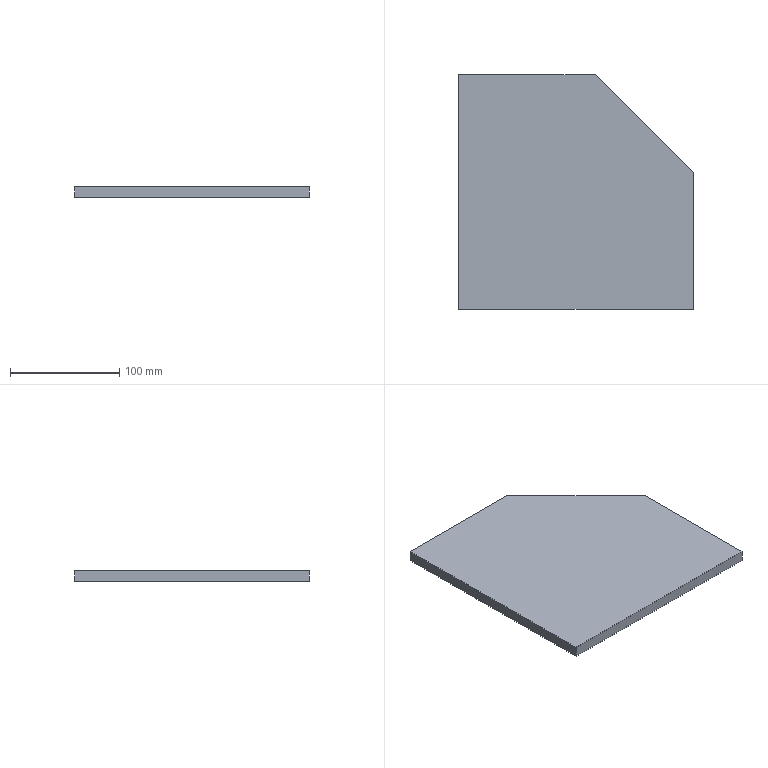Part | STEP file | 03-Reinforcing rib plate | 1 solid | 7 faces | box 215 x 215 x 10 mm | volume 421750 mm3 | plane 7
STEP:
#1=CARTESIAN_POINT('',(0.,0.,0.));
#2=DIRECTION('',(0.,0.,1.));
#3=DIRECTION('',(1.,0.,0.));
#4=AXIS2_PLACEMENT_3D('',#1,#2,#3);
#5=CARTESIAN_POINT('',(0.,0.,0.));
#6=VERTEX_POINT('',#5);
#7=CARTESIAN_POINT('',(0.,-215.,0.));
#8=VERTEX_POINT('',#7);
#9=CARTESIAN_POINT('',(0.,0.,0.));
#10=DIRECTION('',(0.,-1.,0.));
#11=VECTOR('',#10,1.);
#12=LINE('',#9,#11);
#13=CARTESIAN_POINT('',(0.,0.,10.));
#14=DIRECTION('',(1.,0.,0.));
#15=DIRECTION('',(0.,1.,0.));
#16=AXIS2_PLACEMENT_3D('',#13,#14,#15);
#17=PLANE('',#16);
#18=CARTESIAN_POINT('',(0.,-10.));
#19=DIRECTION('',(-1.,0.));
#20=VECTOR('',#19,1.);
#21=LINE('',#18,#20);
#22=(GEOMETRIC_REPRESENTATION_CONTEXT(2)PARAMETRIC_REPRESENTATION_CONTEXT()REPRESENTATION_CONTEXT('',''));
#23=DEFINITIONAL_REPRESENTATION('',(#21),#22);
#24=PCURVE('',#17,#23);
#25=CARTESIAN_POINT('',(0.,0.,0.));
#26=DIRECTION('',(0.,0.,1.));
#27=DIRECTION('',(1.,0.,0.));
#28=AXIS2_PLACEMENT_3D('',#25,#26,#27);
#29=PLANE('',#28);
#30=CARTESIAN_POINT('',(0.,0.));
#31=DIRECTION('',(0.,-1.));
#32=VECTOR('',#31,1.);
#33=LINE('',#30,#32);
#34=(GEOMETRIC_REPRESENTATION_CONTEXT(2)PARAMETRIC_REPRESENTATION_CONTEXT()REPRESENTATION_CONTEXT('',''));
#35=DEFINITIONAL_REPRESENTATION('',(#33),#34);
#36=PCURVE('',#29,#35);
#37=SURFACE_CURVE('',#12,(#24,#36),.PCURVE_S1.);
#38=EDGE_CURVE('',#6,#8,#37,.T.);
#39=ORIENTED_EDGE('',*,*,#38,.T.);
#40=CARTESIAN_POINT('',(0.,-215.,10.));
#41=VERTEX_POINT('',#40);
#42=CARTESIAN_POINT('',(0.,-215.,10.));
#43=DIRECTION('',(0.,0.,-1.));
#44=VECTOR('',#43,1.);
#45=LINE('',#42,#44);
#46=CARTESIAN_POINT('',(-215.,0.));
#47=DIRECTION('',(0.,-1.));
#48=VECTOR('',#47,1.);
#49=LINE('',#46,#48);
#50=(GEOMETRIC_REPRESENTATION_CONTEXT(2)PARAMETRIC_REPRESENTATION_CONTEXT()REPRESENTATION_CONTEXT('',''));
#51=DEFINITIONAL_REPRESENTATION('',(#49),#50);
#52=PCURVE('',#17,#51);
#53=CARTESIAN_POINT('',(0.,-215.,10.));
#54=DIRECTION('',(0.,1.,0.));
#55=DIRECTION('',(0.,0.,1.));
#56=AXIS2_PLACEMENT_3D('',#53,#54,#55);
#57=PLANE('',#56);
#58=CARTESIAN_POINT('',(0.,0.));
#59=DIRECTION('',(-1.,0.));
#60=VECTOR('',#59,1.);
#61=LINE('',#58,#60);
#62=(GEOMETRIC_REPRESENTATION_CONTEXT(2)PARAMETRIC_REPRESENTATION_CONTEXT()REPRESENTATION_CONTEXT('',''));
#63=DEFINITIONAL_REPRESENTATION('',(#61),#62);
#64=PCURVE('',#57,#63);
#65=SURFACE_CURVE('',#45,(#52,#64),.PCURVE_S1.);
#66=EDGE_CURVE('',#41,#8,#65,.T.);
#67=ORIENTED_EDGE('',*,*,#66,.F.);
#68=CARTESIAN_POINT('',(0.,0.,10.));
#69=VERTEX_POINT('',#68);
#70=CARTESIAN_POINT('',(0.,0.,10.));
#71=DIRECTION('',(0.,-1.,0.));
#72=VECTOR('',#71,1.);
#73=LINE('',#70,#72);
#74=CARTESIAN_POINT('',(0.,0.));
#75=DIRECTION('',(-1.,0.));
#76=VECTOR('',#75,1.);
#77=LINE('',#74,#76);
#78=(GEOMETRIC_REPRESENTATION_CONTEXT(2)PARAMETRIC_REPRESENTATION_CONTEXT()REPRESENTATION_CONTEXT('',''));
#79=DEFINITIONAL_REPRESENTATION('',(#77),#78);
#80=PCURVE('',#17,#79);
#81=CARTESIAN_POINT('',(0.,0.,10.));
#82=DIRECTION('',(0.,0.,1.));
#83=DIRECTION('',(1.,0.,0.));
#84=AXIS2_PLACEMENT_3D('',#81,#82,#83);
#85=PLANE('',#84);
#86=CARTESIAN_POINT('',(0.,0.));
#87=DIRECTION('',(0.,-1.));
#88=VECTOR('',#87,1.);
#89=LINE('',#86,#88);
#90=(GEOMETRIC_REPRESENTATION_CONTEXT(2)PARAMETRIC_REPRESENTATION_CONTEXT()REPRESENTATION_CONTEXT('',''));
#91=DEFINITIONAL_REPRESENTATION('',(#89),#90);
#92=PCURVE('',#85,#91);
#93=SURFACE_CURVE('',#73,(#80,#92),.PCURVE_S1.);
#94=EDGE_CURVE('',#69,#41,#93,.T.);
#95=ORIENTED_EDGE('',*,*,#94,.F.);
#96=CARTESIAN_POINT('',(0.,0.,10.));
#97=DIRECTION('',(0.,0.,-1.));
#98=VECTOR('',#97,1.);
#99=LINE('',#96,#98);
#100=CARTESIAN_POINT('',(0.,0.));
#101=DIRECTION('',(0.,-1.));
#102=VECTOR('',#101,1.);
#103=LINE('',#100,#102);
#104=(GEOMETRIC_REPRESENTATION_CONTEXT(2)PARAMETRIC_REPRESENTATION_CONTEXT()REPRESENTATION_CONTEXT('',''));
#105=DEFINITIONAL_REPRESENTATION('',(#103),#104);
#106=PCURVE('',#17,#105);
#107=CARTESIAN_POINT('',(0.,0.,10.));
#108=DIRECTION('',(0.,-1.,0.));
#109=DIRECTION('',(0.,0.,-1.));
#110=AXIS2_PLACEMENT_3D('',#107,#108,#109);
#111=PLANE('',#110);
#112=CARTESIAN_POINT('',(0.,0.));
#113=DIRECTION('',(1.,0.));
#114=VECTOR('',#113,1.);
#115=LINE('',#112,#114);
#116=(GEOMETRIC_REPRESENTATION_CONTEXT(2)PARAMETRIC_REPRESENTATION_CONTEXT()REPRESENTATION_CONTEXT('',''));
#117=DEFINITIONAL_REPRESENTATION('',(#115),#116);
#118=PCURVE('',#111,#117);
#119=SURFACE_CURVE('',#99,(#106,#118),.PCURVE_S1.);
#120=EDGE_CURVE('',#69,#6,#119,.T.);
#121=ORIENTED_EDGE('',*,*,#120,.T.);
#122=EDGE_LOOP('',(#39,#67,#95,#121));
#123=FACE_BOUND('',#122,.T.);
#124=ADVANCED_FACE('',(#123),#17,.F.);
#125=CARTESIAN_POINT('',(215.,-215.,0.));
#126=VERTEX_POINT('',#125);
#127=CARTESIAN_POINT('',(0.,-215.,0.));
#128=DIRECTION('',(1.,0.,0.));
#129=VECTOR('',#128,1.);
#130=LINE('',#127,#129);
#131=CARTESIAN_POINT('',(-10.,0.));
#132=DIRECTION('',(0.,1.));
#133=VECTOR('',#132,1.);
#134=LINE('',#131,#133);
#135=(GEOMETRIC_REPRESENTATION_CONTEXT(2)PARAMETRIC_REPRESENTATION_CONTEXT()REPRESENTATION_CONTEXT('',''));
#136=DEFINITIONAL_REPRESENTATION('',(#134),#135);
#137=PCURVE('',#57,#136);
#138=CARTESIAN_POINT('',(0.,-215.));
#139=DIRECTION('',(1.,0.));
#140=VECTOR('',#139,1.);
#141=LINE('',#138,#140);
#142=(GEOMETRIC_REPRESENTATION_CONTEXT(2)PARAMETRIC_REPRESENTATION_CONTEXT()REPRESENTATION_CONTEXT('',''));
#143=DEFINITIONAL_REPRESENTATION('',(#141),#142);
#144=PCURVE('',#29,#143);
#145=SURFACE_CURVE('',#130,(#137,#144),.PCURVE_S1.);
#146=EDGE_CURVE('',#8,#126,#145,.T.);
#147=ORIENTED_EDGE('',*,*,#146,.T.);
#148=CARTESIAN_POINT('',(215.,-215.,10.));
#149=VERTEX_POINT('',#148);
#150=CARTESIAN_POINT('',(215.,-215.,10.));
#151=DIRECTION('',(0.,0.,-1.));
#152=VECTOR('',#151,1.);
#153=LINE('',#150,#152);
#154=CARTESIAN_POINT('',(0.,215.));
#155=DIRECTION('',(-1.,0.));
#156=VECTOR('',#155,1.);
#157=LINE('',#154,#156);
#158=(GEOMETRIC_REPRESENTATION_CONTEXT(2)PARAMETRIC_REPRESENTATION_CONTEXT()REPRESENTATION_CONTEXT('',''));
#159=DEFINITIONAL_REPRESENTATION('',(#157),#158);
#160=PCURVE('',#57,#159);
#161=CARTESIAN_POINT('',(215.,-90.,10.));
#162=DIRECTION('',(-1.,0.,0.));
#163=DIRECTION('',(0.,-1.,0.));
#164=AXIS2_PLACEMENT_3D('',#161,#162,#163);
#165=PLANE('',#164);
#166=CARTESIAN_POINT('',(125.,0.));
#167=DIRECTION('',(0.,-1.));
#168=VECTOR('',#167,1.);
#169=LINE('',#166,#168);
#170=(GEOMETRIC_REPRESENTATION_CONTEXT(2)PARAMETRIC_REPRESENTATION_CONTEXT()REPRESENTATION_CONTEXT('',''));
#171=DEFINITIONAL_REPRESENTATION('',(#169),#170);
#172=PCURVE('',#165,#171);
#173=SURFACE_CURVE('',#153,(#160,#172),.PCURVE_S1.);
#174=EDGE_CURVE('',#149,#126,#173,.T.);
#175=ORIENTED_EDGE('',*,*,#174,.F.);
#176=CARTESIAN_POINT('',(0.,-215.,10.));
#177=DIRECTION('',(1.,0.,0.));
#178=VECTOR('',#177,1.);
#179=LINE('',#176,#178);
#180=CARTESIAN_POINT('',(0.,0.));
#181=DIRECTION('',(0.,1.));
#182=VECTOR('',#181,1.);
#183=LINE('',#180,#182);
#184=(GEOMETRIC_REPRESENTATION_CONTEXT(2)PARAMETRIC_REPRESENTATION_CONTEXT()REPRESENTATION_CONTEXT('',''));
#185=DEFINITIONAL_REPRESENTATION('',(#183),#184);
#186=PCURVE('',#57,#185);
#187=CARTESIAN_POINT('',(0.,-215.));
#188=DIRECTION('',(1.,0.));
#189=VECTOR('',#188,1.);
#190=LINE('',#187,#189);
#191=(GEOMETRIC_REPRESENTATION_CONTEXT(2)PARAMETRIC_REPRESENTATION_CONTEXT()REPRESENTATION_CONTEXT('',''));
#192=DEFINITIONAL_REPRESENTATION('',(#190),#191);
#193=PCURVE('',#85,#192);
#194=SURFACE_CURVE('',#179,(#186,#193),.PCURVE_S1.);
#195=EDGE_CURVE('',#41,#149,#194,.T.);
#196=ORIENTED_EDGE('',*,*,#195,.F.);
#197=ORIENTED_EDGE('',*,*,#66,.T.);
#198=EDGE_LOOP('',(#147,#175,#196,#197));
#199=FACE_BOUND('',#198,.T.);
#200=ADVANCED_FACE('',(#199),#57,.F.);
#201=CARTESIAN_POINT('',(215.,-90.,0.));
#202=VERTEX_POINT('',#201);
#203=CARTESIAN_POINT('',(215.,-90.,0.));
#204=DIRECTION('',(0.,1.,0.));
#205=VECTOR('',#204,1.);
#206=LINE('',#203,#205);
#207=CARTESIAN_POINT('',(0.,-10.));
#208=DIRECTION('',(-1.,0.));
#209=VECTOR('',#208,1.);
#210=LINE('',#207,#209);
#211=(GEOMETRIC_REPRESENTATION_CONTEXT(2)PARAMETRIC_REPRESENTATION_CONTEXT()REPRESENTATION_CONTEXT('',''));
#212=DEFINITIONAL_REPRESENTATION('',(#210),#211);
#213=PCURVE('',#165,#212);
#214=CARTESIAN_POINT('',(215.,-90.));
#215=DIRECTION('',(0.,1.));
#216=VECTOR('',#215,1.);
#217=LINE('',#214,#216);
#218=(GEOMETRIC_REPRESENTATION_CONTEXT(2)PARAMETRIC_REPRESENTATION_CONTEXT()REPRESENTATION_CONTEXT('',''));
#219=DEFINITIONAL_REPRESENTATION('',(#217),#218);
#220=PCURVE('',#29,#219);
#221=SURFACE_CURVE('',#206,(#213,#220),.PCURVE_S1.);
#222=EDGE_CURVE('',#126,#202,#221,.T.);
#223=ORIENTED_EDGE('',*,*,#222,.T.);
#224=CARTESIAN_POINT('',(215.,-90.,10.));
#225=VERTEX_POINT('',#224);
#226=CARTESIAN_POINT('',(215.,-90.,10.));
#227=DIRECTION('',(0.,0.,-1.));
#228=VECTOR('',#227,1.);
#229=LINE('',#226,#228);
#230=CARTESIAN_POINT('',(0.,0.));
#231=DIRECTION('',(0.,-1.));
#232=VECTOR('',#231,1.);
#233=LINE('',#230,#232);
#234=(GEOMETRIC_REPRESENTATION_CONTEXT(2)PARAMETRIC_REPRESENTATION_CONTEXT()REPRESENTATION_CONTEXT('',''));
#235=DEFINITIONAL_REPRESENTATION('',(#233),#234);
#236=PCURVE('',#165,#235);
#237=CARTESIAN_POINT('',(125.,0.,10.));
#238=DIRECTION('',(-0.7071,-0.7071,0.));
#239=DIRECTION('',(0.7071,-0.7071,0.));
#240=AXIS2_PLACEMENT_3D('',#237,#238,#239);
#241=PLANE('',#240);
#242=CARTESIAN_POINT('',(127.279,0.));
#243=DIRECTION('',(0.,-1.));
#244=VECTOR('',#243,1.);
#245=LINE('',#242,#244);
#246=(GEOMETRIC_REPRESENTATION_CONTEXT(2)PARAMETRIC_REPRESENTATION_CONTEXT()REPRESENTATION_CONTEXT('',''));
#247=DEFINITIONAL_REPRESENTATION('',(#245),#246);
#248=PCURVE('',#241,#247);
#249=SURFACE_CURVE('',#229,(#236,#248),.PCURVE_S1.);
#250=EDGE_CURVE('',#225,#202,#249,.T.);
#251=ORIENTED_EDGE('',*,*,#250,.F.);
#252=CARTESIAN_POINT('',(215.,-90.,10.));
#253=DIRECTION('',(0.,1.,0.));
#254=VECTOR('',#253,1.);
#255=LINE('',#252,#254);
#256=CARTESIAN_POINT('',(0.,0.));
#257=DIRECTION('',(-1.,0.));
#258=VECTOR('',#257,1.);
#259=LINE('',#256,#258);
#260=(GEOMETRIC_REPRESENTATION_CONTEXT(2)PARAMETRIC_REPRESENTATION_CONTEXT()REPRESENTATION_CONTEXT('',''));
#261=DEFINITIONAL_REPRESENTATION('',(#259),#260);
#262=PCURVE('',#165,#261);
#263=CARTESIAN_POINT('',(215.,-90.));
#264=DIRECTION('',(0.,1.));
#265=VECTOR('',#264,1.);
#266=LINE('',#263,#265);
#267=(GEOMETRIC_REPRESENTATION_CONTEXT(2)PARAMETRIC_REPRESENTATION_CONTEXT()REPRESENTATION_CONTEXT('',''));
#268=DEFINITIONAL_REPRESENTATION('',(#266),#267);
#269=PCURVE('',#85,#268);
#270=SURFACE_CURVE('',#255,(#262,#269),.PCURVE_S1.);
#271=EDGE_CURVE('',#149,#225,#270,.T.);
#272=ORIENTED_EDGE('',*,*,#271,.F.);
#273=ORIENTED_EDGE('',*,*,#174,.T.);
#274=EDGE_LOOP('',(#223,#251,#272,#273));
#275=FACE_BOUND('',#274,.T.);
#276=ADVANCED_FACE('',(#275),#165,.F.);
#277=CARTESIAN_POINT('',(125.,0.,0.));
#278=VERTEX_POINT('',#277);
#279=CARTESIAN_POINT('',(125.,0.,0.));
#280=DIRECTION('',(-0.7071,0.7071,0.));
#281=VECTOR('',#280,1.);
#282=LINE('',#279,#281);
#283=CARTESIAN_POINT('',(0.,-10.));
#284=DIRECTION('',(-1.,0.));
#285=VECTOR('',#284,1.);
#286=LINE('',#283,#285);
#287=(GEOMETRIC_REPRESENTATION_CONTEXT(2)PARAMETRIC_REPRESENTATION_CONTEXT()REPRESENTATION_CONTEXT('',''));
#288=DEFINITIONAL_REPRESENTATION('',(#286),#287);
#289=PCURVE('',#241,#288);
#290=CARTESIAN_POINT('',(125.,0.));
#291=DIRECTION('',(-0.7071,0.7071));
#292=VECTOR('',#291,1.);
#293=LINE('',#290,#292);
#294=(GEOMETRIC_REPRESENTATION_CONTEXT(2)PARAMETRIC_REPRESENTATION_CONTEXT()REPRESENTATION_CONTEXT('',''));
#295=DEFINITIONAL_REPRESENTATION('',(#293),#294);
#296=PCURVE('',#29,#295);
#297=SURFACE_CURVE('',#282,(#289,#296),.PCURVE_S1.);
#298=EDGE_CURVE('',#202,#278,#297,.T.);
#299=ORIENTED_EDGE('',*,*,#298,.T.);
#300=CARTESIAN_POINT('',(125.,0.,10.));
#301=VERTEX_POINT('',#300);
#302=CARTESIAN_POINT('',(125.,0.,10.));
#303=DIRECTION('',(0.,0.,-1.));
#304=VECTOR('',#303,1.);
#305=LINE('',#302,#304);
#306=CARTESIAN_POINT('',(0.,0.));
#307=DIRECTION('',(0.,-1.));
#308=VECTOR('',#307,1.);
#309=LINE('',#306,#308);
#310=(GEOMETRIC_REPRESENTATION_CONTEXT(2)PARAMETRIC_REPRESENTATION_CONTEXT()REPRESENTATION_CONTEXT('',''));
#311=DEFINITIONAL_REPRESENTATION('',(#309),#310);
#312=PCURVE('',#241,#311);
#313=CARTESIAN_POINT('',(0.,125.));
#314=DIRECTION('',(1.,0.));
#315=VECTOR('',#314,1.);
#316=LINE('',#313,#315);
#317=(GEOMETRIC_REPRESENTATION_CONTEXT(2)PARAMETRIC_REPRESENTATION_CONTEXT()REPRESENTATION_CONTEXT('',''));
#318=DEFINITIONAL_REPRESENTATION('',(#316),#317);
#319=PCURVE('',#111,#318);
#320=SURFACE_CURVE('',#305,(#312,#319),.PCURVE_S1.);
#321=EDGE_CURVE('',#301,#278,#320,.T.);
#322=ORIENTED_EDGE('',*,*,#321,.F.);
#323=CARTESIAN_POINT('',(125.,0.,10.));
#324=DIRECTION('',(-0.7071,0.7071,0.));
#325=VECTOR('',#324,1.);
#326=LINE('',#323,#325);
#327=CARTESIAN_POINT('',(0.,0.));
#328=DIRECTION('',(-1.,0.));
#329=VECTOR('',#328,1.);
#330=LINE('',#327,#329);
#331=(GEOMETRIC_REPRESENTATION_CONTEXT(2)PARAMETRIC_REPRESENTATION_CONTEXT()REPRESENTATION_CONTEXT('',''));
#332=DEFINITIONAL_REPRESENTATION('',(#330),#331);
#333=PCURVE('',#241,#332);
#334=CARTESIAN_POINT('',(125.,0.));
#335=DIRECTION('',(-0.7071,0.7071));
#336=VECTOR('',#335,1.);
#337=LINE('',#334,#336);
#338=(GEOMETRIC_REPRESENTATION_CONTEXT(2)PARAMETRIC_REPRESENTATION_CONTEXT()REPRESENTATION_CONTEXT('',''));
#339=DEFINITIONAL_REPRESENTATION('',(#337),#338);
#340=PCURVE('',#85,#339);
#341=SURFACE_CURVE('',#326,(#333,#340),.PCURVE_S1.);
#342=EDGE_CURVE('',#225,#301,#341,.T.);
#343=ORIENTED_EDGE('',*,*,#342,.F.);
#344=ORIENTED_EDGE('',*,*,#250,.T.);
#345=EDGE_LOOP('',(#299,#322,#343,#344));
#346=FACE_BOUND('',#345,.T.);
#347=ADVANCED_FACE('',(#346),#241,.F.);
#348=CARTESIAN_POINT('',(0.,0.,0.));
#349=DIRECTION('',(-1.,0.,0.));
#350=VECTOR('',#349,1.);
#351=LINE('',#348,#350);
#352=CARTESIAN_POINT('',(10.,0.));
#353=DIRECTION('',(0.,-1.));
#354=VECTOR('',#353,1.);
#355=LINE('',#352,#354);
#356=(GEOMETRIC_REPRESENTATION_CONTEXT(2)PARAMETRIC_REPRESENTATION_CONTEXT()REPRESENTATION_CONTEXT('',''));
#357=DEFINITIONAL_REPRESENTATION('',(#355),#356);
#358=PCURVE('',#111,#357);
#359=CARTESIAN_POINT('',(0.,0.));
#360=DIRECTION('',(-1.,0.));
#361=VECTOR('',#360,1.);
#362=LINE('',#359,#361);
#363=(GEOMETRIC_REPRESENTATION_CONTEXT(2)PARAMETRIC_REPRESENTATION_CONTEXT()REPRESENTATION_CONTEXT('',''));
#364=DEFINITIONAL_REPRESENTATION('',(#362),#363);
#365=PCURVE('',#29,#364);
#366=SURFACE_CURVE('',#351,(#358,#365),.PCURVE_S1.);
#367=EDGE_CURVE('',#278,#6,#366,.T.);
#368=ORIENTED_EDGE('',*,*,#367,.T.);
#369=ORIENTED_EDGE('',*,*,#120,.F.);
#370=CARTESIAN_POINT('',(0.,0.,10.));
#371=DIRECTION('',(-1.,0.,0.));
#372=VECTOR('',#371,1.);
#373=LINE('',#370,#372);
#374=CARTESIAN_POINT('',(0.,0.));
#375=DIRECTION('',(0.,-1.));
#376=VECTOR('',#375,1.);
#377=LINE('',#374,#376);
#378=(GEOMETRIC_REPRESENTATION_CONTEXT(2)PARAMETRIC_REPRESENTATION_CONTEXT()REPRESENTATION_CONTEXT('',''));
#379=DEFINITIONAL_REPRESENTATION('',(#377),#378);
#380=PCURVE('',#111,#379);
#381=CARTESIAN_POINT('',(0.,0.));
#382=DIRECTION('',(-1.,0.));
#383=VECTOR('',#382,1.);
#384=LINE('',#381,#383);
#385=(GEOMETRIC_REPRESENTATION_CONTEXT(2)PARAMETRIC_REPRESENTATION_CONTEXT()REPRESENTATION_CONTEXT('',''));
#386=DEFINITIONAL_REPRESENTATION('',(#384),#385);
#387=PCURVE('',#85,#386);
#388=SURFACE_CURVE('',#373,(#380,#387),.PCURVE_S1.);
#389=EDGE_CURVE('',#301,#69,#388,.T.);
#390=ORIENTED_EDGE('',*,*,#389,.F.);
#391=ORIENTED_EDGE('',*,*,#321,.T.);
#392=EDGE_LOOP('',(#368,#369,#390,#391));
#393=FACE_BOUND('',#392,.T.);
#394=ADVANCED_FACE('',(#393),#111,.F.);
#395=ORIENTED_EDGE('',*,*,#94,.T.);
#396=ORIENTED_EDGE('',*,*,#195,.T.);
#397=ORIENTED_EDGE('',*,*,#271,.T.);
#398=ORIENTED_EDGE('',*,*,#342,.T.);
#399=ORIENTED_EDGE('',*,*,#389,.T.);
#400=EDGE_LOOP('',(#395,#396,#397,#398,#399));
#401=FACE_BOUND('',#400,.T.);
#402=ADVANCED_FACE('',(#401),#85,.T.);
#403=ORIENTED_EDGE('',*,*,#38,.F.);
#404=ORIENTED_EDGE('',*,*,#367,.F.);
#405=ORIENTED_EDGE('',*,*,#298,.F.);
#406=ORIENTED_EDGE('',*,*,#222,.F.);
#407=ORIENTED_EDGE('',*,*,#146,.F.);
#408=EDGE_LOOP('',(#403,#404,#405,#406,#407));
#409=FACE_BOUND('',#408,.T.);
#410=ADVANCED_FACE('',(#409),#29,.F.);
#411=CLOSED_SHELL('',(#124,#200,#276,#347,#394,#402,#410));
#412=MANIFOLD_SOLID_BREP('',#411);
#413=(LENGTH_UNIT()NAMED_UNIT(*)SI_UNIT(.MILLI.,.METRE.));
#414=UNCERTAINTY_MEASURE_WITH_UNIT(LENGTH_MEASURE(0.0000001),#413,'','');
#415=(NAMED_UNIT(*)PLANE_ANGLE_UNIT()SI_UNIT($,.RADIAN.));
#416=(NAMED_UNIT(*)SI_UNIT($,.STERADIAN.)SOLID_ANGLE_UNIT());
#417=(GEOMETRIC_REPRESENTATION_CONTEXT(3)GLOBAL_UNCERTAINTY_ASSIGNED_CONTEXT((#414))GLOBAL_UNIT_ASSIGNED_CONTEXT((#413,#415,#416))REPRESENTATION_CONTEXT('',''));
#418=ADVANCED_BREP_SHAPE_REPRESENTATION('',(#4,#412),#417);